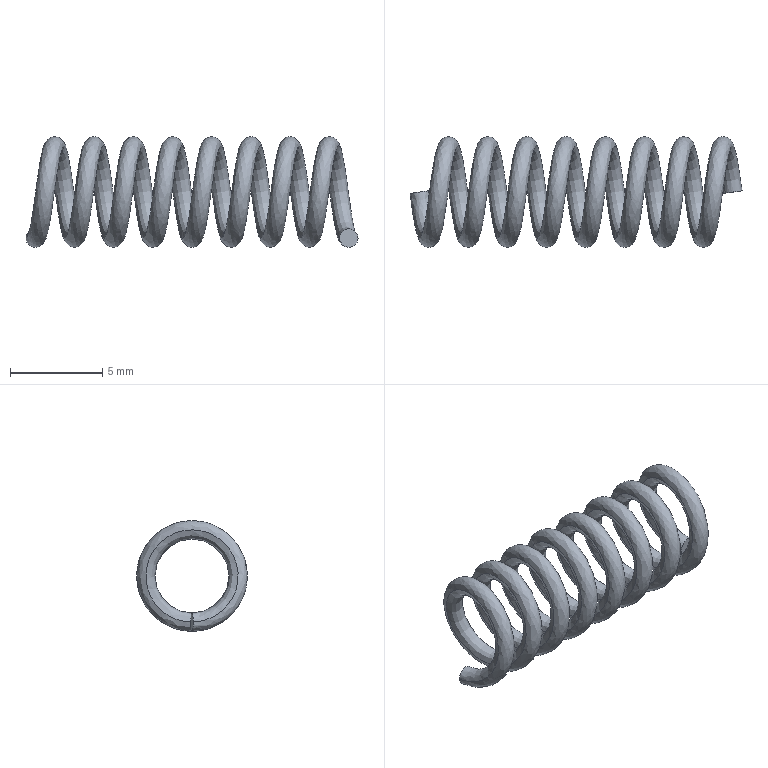Part | SolidWorks | features BaseBody 1 | 1 solid | 4 faces | box 17.991 x 6 x 6 mm | volume 99.073 mm3 | spline 2 | plane 2